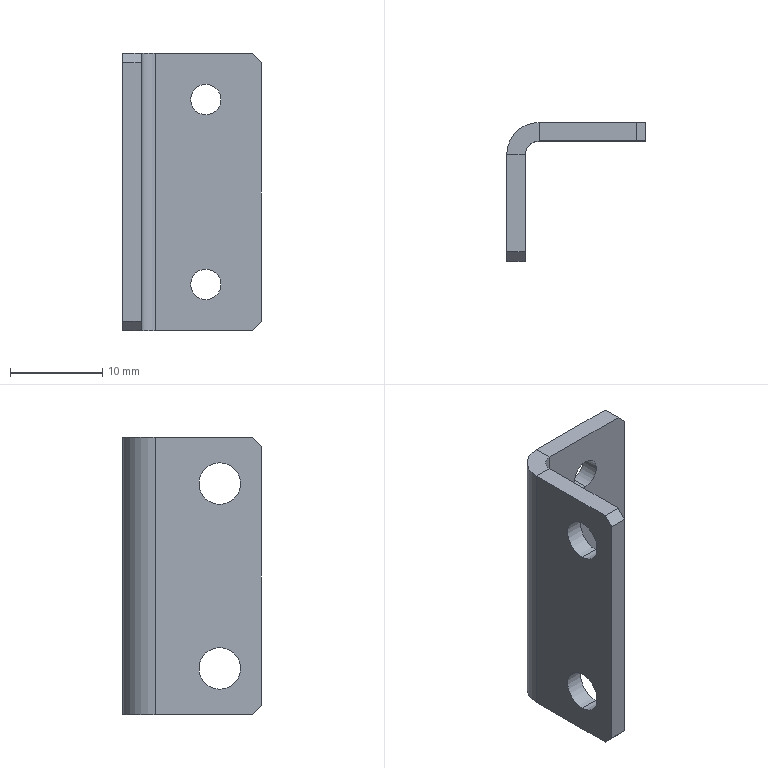Part | SolidWorks | features HoleWzd 2, Chamfer 1, FlatPattern 1, SMBaseFlange 1, SheetMetal 1 | 1 solid | 26 faces | box 15 x 15 x 30 mm | volume 1514 mm3 | plane 16 | cylinder 10 | commonest cylinder face diameters 3.3 x4 4.5 x4 3 x1 7 x1
STEP:
#1=CARTESIAN_POINT('',(2.,4.5,-12.25));
#2=VERTEX_POINT('',#1);
#3=CARTESIAN_POINT('',(2.,4.5,-7.75));
#4=VERTEX_POINT('',#3);
#5=CARTESIAN_POINT('',(2.,4.5,-10.));
#6=DIRECTION('',(-1.,0.,0.));
#7=DIRECTION('',(0.,0.,1.));
#8=AXIS2_PLACEMENT_3D('',#5,#6,#7);
#9=CIRCLE('',#8,2.25);
#10=EDGE_CURVE('',#2,#4,#9,.T.);
#11=ORIENTED_EDGE('',*,*,#10,.F.);
#12=CARTESIAN_POINT('',(0.,4.5,-12.25));
#13=VERTEX_POINT('',#12);
#14=CARTESIAN_POINT('',(0.,4.5,-12.25));
#15=DIRECTION('',(-1.,0.,0.));
#16=VECTOR('',#15,1000.);
#17=LINE('',#14,#16);
#18=EDGE_CURVE('',#2,#13,#17,.T.);
#19=ORIENTED_EDGE('',*,*,#18,.T.);
#20=CARTESIAN_POINT('',(0.,4.5,-7.75));
#21=VERTEX_POINT('',#20);
#22=CARTESIAN_POINT('',(0.,4.5,-10.));
#23=DIRECTION('',(-1.,0.,0.));
#24=DIRECTION('',(0.,0.,1.));
#25=AXIS2_PLACEMENT_3D('',#22,#23,#24);
#26=CIRCLE('',#25,2.25);
#27=EDGE_CURVE('',#13,#21,#26,.T.);
#28=ORIENTED_EDGE('',*,*,#27,.T.);
#29=CARTESIAN_POINT('',(0.,4.5,-7.75));
#30=DIRECTION('',(-1.,0.,0.));
#31=VECTOR('',#30,1000.);
#32=LINE('',#29,#31);
#33=EDGE_CURVE('',#4,#21,#32,.T.);
#34=ORIENTED_EDGE('',*,*,#33,.F.);
#35=EDGE_LOOP('',(#11,#19,#28,#34));
#36=FACE_OUTER_BOUND('',#35,.T.);
#37=CARTESIAN_POINT('',(0.,4.5,-10.));
#38=DIRECTION('',(-1.,0.,0.));
#39=DIRECTION('',(0.,0.,1.));
#40=AXIS2_PLACEMENT_3D('',#37,#38,#39);
#41=CYLINDRICAL_SURFACE('',#40,2.25);
#42=ADVANCED_FACE('',(#36),#41,.F.);
#43=CARTESIAN_POINT('',(2.,4.5,7.75));
#44=VERTEX_POINT('',#43);
#45=CARTESIAN_POINT('',(2.,4.5,12.25));
#46=VERTEX_POINT('',#45);
#47=CARTESIAN_POINT('',(2.,4.5,10.));
#48=DIRECTION('',(-1.,0.,0.));
#49=DIRECTION('',(0.,0.,1.));
#50=AXIS2_PLACEMENT_3D('',#47,#48,#49);
#51=CIRCLE('',#50,2.25);
#52=EDGE_CURVE('',#44,#46,#51,.T.);
#53=ORIENTED_EDGE('',*,*,#52,.F.);
#54=CARTESIAN_POINT('',(0.,4.5,7.75));
#55=VERTEX_POINT('',#54);
#56=CARTESIAN_POINT('',(0.,4.5,7.75));
#57=DIRECTION('',(-1.,0.,0.));
#58=VECTOR('',#57,1000.);
#59=LINE('',#56,#58);
#60=EDGE_CURVE('',#44,#55,#59,.T.);
#61=ORIENTED_EDGE('',*,*,#60,.T.);
#62=CARTESIAN_POINT('',(0.,4.5,12.25));
#63=VERTEX_POINT('',#62);
#64=CARTESIAN_POINT('',(0.,4.5,10.));
#65=DIRECTION('',(-1.,0.,0.));
#66=DIRECTION('',(0.,0.,1.));
#67=AXIS2_PLACEMENT_3D('',#64,#65,#66);
#68=CIRCLE('',#67,2.25);
#69=EDGE_CURVE('',#55,#63,#68,.T.);
#70=ORIENTED_EDGE('',*,*,#69,.T.);
#71=CARTESIAN_POINT('',(0.,4.5,12.25));
#72=DIRECTION('',(-1.,0.,0.));
#73=VECTOR('',#72,1000.);
#74=LINE('',#71,#73);
#75=EDGE_CURVE('',#46,#63,#74,.T.);
#76=ORIENTED_EDGE('',*,*,#75,.F.);
#77=EDGE_LOOP('',(#53,#61,#70,#76));
#78=FACE_OUTER_BOUND('',#77,.T.);
#79=CARTESIAN_POINT('',(0.,4.5,10.));
#80=DIRECTION('',(-1.,0.,0.));
#81=DIRECTION('',(0.,0.,1.));
#82=AXIS2_PLACEMENT_3D('',#79,#80,#81);
#83=CYLINDRICAL_SURFACE('',#82,2.25);
#84=ADVANCED_FACE('',(#78),#83,.F.);
#85=CARTESIAN_POINT('',(9.,13.,-11.65));
#86=VERTEX_POINT('',#85);
#87=CARTESIAN_POINT('',(9.,13.,-8.35));
#88=VERTEX_POINT('',#87);
#89=CARTESIAN_POINT('',(9.,13.,-10.));
#90=DIRECTION('',(0.,1.,0.));
#91=DIRECTION('',(0.,0.,1.));
#92=AXIS2_PLACEMENT_3D('',#89,#90,#91);
#93=CIRCLE('',#92,1.65);
#94=EDGE_CURVE('',#86,#88,#93,.T.);
#95=ORIENTED_EDGE('',*,*,#94,.F.);
#96=CARTESIAN_POINT('',(9.,15.,-11.65));
#97=VERTEX_POINT('',#96);
#98=CARTESIAN_POINT('',(9.,15.,-11.65));
#99=DIRECTION('',(0.,1.,0.));
#100=VECTOR('',#99,1000.);
#101=LINE('',#98,#100);
#102=EDGE_CURVE('',#86,#97,#101,.T.);
#103=ORIENTED_EDGE('',*,*,#102,.T.);
#104=CARTESIAN_POINT('',(9.,15.,-8.35));
#105=VERTEX_POINT('',#104);
#106=CARTESIAN_POINT('',(9.,15.,-10.));
#107=DIRECTION('',(0.,1.,0.));
#108=DIRECTION('',(0.,0.,1.));
#109=AXIS2_PLACEMENT_3D('',#106,#107,#108);
#110=CIRCLE('',#109,1.65);
#111=EDGE_CURVE('',#97,#105,#110,.T.);
#112=ORIENTED_EDGE('',*,*,#111,.T.);
#113=CARTESIAN_POINT('',(9.,15.,-8.35));
#114=DIRECTION('',(0.,1.,0.));
#115=VECTOR('',#114,1000.);
#116=LINE('',#113,#115);
#117=EDGE_CURVE('',#88,#105,#116,.T.);
#118=ORIENTED_EDGE('',*,*,#117,.F.);
#119=EDGE_LOOP('',(#95,#103,#112,#118));
#120=FACE_OUTER_BOUND('',#119,.T.);
#121=CARTESIAN_POINT('',(9.,15.,-10.));
#122=DIRECTION('',(0.,1.,0.));
#123=DIRECTION('',(0.,0.,1.));
#124=AXIS2_PLACEMENT_3D('',#121,#122,#123);
#125=CYLINDRICAL_SURFACE('',#124,1.65);
#126=ADVANCED_FACE('',(#120),#125,.F.);
#127=CARTESIAN_POINT('',(9.,13.,8.35));
#128=VERTEX_POINT('',#127);
#129=CARTESIAN_POINT('',(9.,13.,11.65));
#130=VERTEX_POINT('',#129);
#131=CARTESIAN_POINT('',(9.,13.,10.));
#132=DIRECTION('',(0.,1.,0.));
#133=DIRECTION('',(0.,0.,1.));
#134=AXIS2_PLACEMENT_3D('',#131,#132,#133);
#135=CIRCLE('',#134,1.65);
#136=EDGE_CURVE('',#128,#130,#135,.T.);
#137=ORIENTED_EDGE('',*,*,#136,.F.);
#138=CARTESIAN_POINT('',(9.,15.,8.35));
#139=VERTEX_POINT('',#138);
#140=CARTESIAN_POINT('',(9.,15.,8.35));
#141=DIRECTION('',(0.,1.,0.));
#142=VECTOR('',#141,1000.);
#143=LINE('',#140,#142);
#144=EDGE_CURVE('',#128,#139,#143,.T.);
#145=ORIENTED_EDGE('',*,*,#144,.T.);
#146=CARTESIAN_POINT('',(9.,15.,11.65));
#147=VERTEX_POINT('',#146);
#148=CARTESIAN_POINT('',(9.,15.,10.));
#149=DIRECTION('',(0.,1.,0.));
#150=DIRECTION('',(0.,0.,1.));
#151=AXIS2_PLACEMENT_3D('',#148,#149,#150);
#152=CIRCLE('',#151,1.65);
#153=EDGE_CURVE('',#139,#147,#152,.T.);
#154=ORIENTED_EDGE('',*,*,#153,.T.);
#155=CARTESIAN_POINT('',(9.,15.,11.65));
#156=DIRECTION('',(0.,1.,0.));
#157=VECTOR('',#156,1000.);
#158=LINE('',#155,#157);
#159=EDGE_CURVE('',#130,#147,#158,.T.);
#160=ORIENTED_EDGE('',*,*,#159,.F.);
#161=EDGE_LOOP('',(#137,#145,#154,#160));
#162=FACE_OUTER_BOUND('',#161,.T.);
#163=CARTESIAN_POINT('',(9.,15.,10.));
#164=DIRECTION('',(0.,1.,0.));
#165=DIRECTION('',(0.,0.,1.));
#166=AXIS2_PLACEMENT_3D('',#163,#164,#165);
#167=CYLINDRICAL_SURFACE('',#166,1.65);
#168=ADVANCED_FACE('',(#162),#167,.F.);
#169=CARTESIAN_POINT('',(3.5,15.,15.));
#170=VERTEX_POINT('',#169);
#171=CARTESIAN_POINT('',(3.5,13.,15.));
#172=VERTEX_POINT('',#171);
#173=CARTESIAN_POINT('',(3.5,15.,15.));
#174=DIRECTION('',(0.,-1.,0.));
#175=VECTOR('',#174,1000.);
#176=LINE('',#173,#175);
#177=EDGE_CURVE('',#170,#172,#176,.T.);
#178=ORIENTED_EDGE('',*,*,#177,.F.);
#179=CARTESIAN_POINT('',(0.,11.5,15.));
#180=VERTEX_POINT('',#179);
#181=CARTESIAN_POINT('',(3.5,11.5,15.));
#182=DIRECTION('',(0.,0.,-1.));
#183=DIRECTION('',(1.,0.,0.));
#184=AXIS2_PLACEMENT_3D('',#181,#182,#183);
#185=CIRCLE('',#184,3.5);
#186=EDGE_CURVE('',#180,#170,#185,.T.);
#187=ORIENTED_EDGE('',*,*,#186,.F.);
#188=CARTESIAN_POINT('',(2.,11.5,15.));
#189=VERTEX_POINT('',#188);
#190=CARTESIAN_POINT('',(2.,11.5,15.));
#191=DIRECTION('',(-1.,0.,0.));
#192=VECTOR('',#191,1000.);
#193=LINE('',#190,#192);
#194=EDGE_CURVE('',#189,#180,#193,.T.);
#195=ORIENTED_EDGE('',*,*,#194,.F.);
#196=CARTESIAN_POINT('',(3.5,11.5,15.));
#197=DIRECTION('',(0.,0.,-1.));
#198=DIRECTION('',(1.,0.,0.));
#199=AXIS2_PLACEMENT_3D('',#196,#197,#198);
#200=CIRCLE('',#199,1.5);
#201=EDGE_CURVE('',#189,#172,#200,.T.);
#202=ORIENTED_EDGE('',*,*,#201,.T.);
#203=EDGE_LOOP('',(#178,#187,#195,#202));
#204=FACE_OUTER_BOUND('',#203,.T.);
#205=CARTESIAN_POINT('',(3.5,15.,15.));
#206=DIRECTION('',(0.,0.,1.));
#207=DIRECTION('',(1.,0.,0.));
#208=AXIS2_PLACEMENT_3D('',#205,#206,#207);
#209=PLANE('',#208);
#210=ADVANCED_FACE('',(#204),#209,.T.);
#211=CARTESIAN_POINT('',(14.,13.,15.));
#212=VERTEX_POINT('',#211);
#213=CARTESIAN_POINT('',(0.,13.,15.));
#214=DIRECTION('',(1.,0.,0.));
#215=VECTOR('',#214,1000.);
#216=LINE('',#213,#215);
#217=EDGE_CURVE('',#172,#212,#216,.T.);
#218=ORIENTED_EDGE('',*,*,#217,.T.);
#219=CARTESIAN_POINT('',(14.,15.,15.));
#220=VERTEX_POINT('',#219);
#221=CARTESIAN_POINT('',(14.,11.5,15.));
#222=DIRECTION('',(0.,1.,0.));
#223=VECTOR('',#222,1000.);
#224=LINE('',#221,#223);
#225=EDGE_CURVE('',#212,#220,#224,.T.);
#226=ORIENTED_EDGE('',*,*,#225,.T.);
#227=CARTESIAN_POINT('',(0.,15.,15.));
#228=DIRECTION('',(1.,0.,0.));
#229=VECTOR('',#228,1000.);
#230=LINE('',#227,#229);
#231=EDGE_CURVE('',#170,#220,#230,.T.);
#232=ORIENTED_EDGE('',*,*,#231,.F.);
#233=ORIENTED_EDGE('',*,*,#177,.T.);
#234=EDGE_LOOP('',(#218,#226,#232,#233));
#235=FACE_OUTER_BOUND('',#234,.T.);
#236=CARTESIAN_POINT('',(2.,11.5,15.));
#237=DIRECTION('',(0.,0.,1.));
#238=DIRECTION('',(1.,0.,0.));
#239=AXIS2_PLACEMENT_3D('',#236,#237,#238);
#240=PLANE('',#239);
#241=ADVANCED_FACE('',(#235),#240,.T.);
#242=CARTESIAN_POINT('',(0.,11.5,-15.));
#243=VERTEX_POINT('',#242);
#244=CARTESIAN_POINT('',(2.,11.5,-15.));
#245=VERTEX_POINT('',#244);
#246=CARTESIAN_POINT('',(0.,11.5,-15.));
#247=DIRECTION('',(1.,0.,0.));
#248=VECTOR('',#247,1000.);
#249=LINE('',#246,#248);
#250=EDGE_CURVE('',#243,#245,#249,.T.);
#251=ORIENTED_EDGE('',*,*,#250,.F.);
#252=CARTESIAN_POINT('',(3.5,15.,-15.));
#253=VERTEX_POINT('',#252);
#254=CARTESIAN_POINT('',(3.5,11.5,-15.));
#255=DIRECTION('',(0.,0.,-1.));
#256=DIRECTION('',(1.,0.,0.));
#257=AXIS2_PLACEMENT_3D('',#254,#255,#256);
#258=CIRCLE('',#257,3.5);
#259=EDGE_CURVE('',#243,#253,#258,.T.);
#260=ORIENTED_EDGE('',*,*,#259,.T.);
#261=CARTESIAN_POINT('',(3.5,13.,-15.));
#262=VERTEX_POINT('',#261);
#263=CARTESIAN_POINT('',(3.5,13.,-15.));
#264=DIRECTION('',(0.,1.,0.));
#265=VECTOR('',#264,1000.);
#266=LINE('',#263,#265);
#267=EDGE_CURVE('',#262,#253,#266,.T.);
#268=ORIENTED_EDGE('',*,*,#267,.F.);
#269=CARTESIAN_POINT('',(3.5,11.5,-15.));
#270=DIRECTION('',(0.,0.,-1.));
#271=DIRECTION('',(1.,0.,0.));
#272=AXIS2_PLACEMENT_3D('',#269,#270,#271);
#273=CIRCLE('',#272,1.5);
#274=EDGE_CURVE('',#245,#262,#273,.T.);
#275=ORIENTED_EDGE('',*,*,#274,.F.);
#276=EDGE_LOOP('',(#251,#260,#268,#275));
#277=FACE_OUTER_BOUND('',#276,.T.);
#278=CARTESIAN_POINT('',(0.,11.5,-15.));
#279=DIRECTION('',(0.,0.,-1.));
#280=DIRECTION('',(-1.,0.,0.));
#281=AXIS2_PLACEMENT_3D('',#278,#279,#280);
#282=PLANE('',#281);
#283=ADVANCED_FACE('',(#277),#282,.T.);
#284=CARTESIAN_POINT('',(2.,1.,-15.));
#285=VERTEX_POINT('',#284);
#286=CARTESIAN_POINT('',(2.,0.,-15.));
#287=DIRECTION('',(0.,1.,0.));
#288=VECTOR('',#287,1000.);
#289=LINE('',#286,#288);
#290=EDGE_CURVE('',#285,#245,#289,.T.);
#291=ORIENTED_EDGE('',*,*,#290,.F.);
#292=CARTESIAN_POINT('',(0.,1.,-15.));
#293=VERTEX_POINT('',#292);
#294=CARTESIAN_POINT('',(3.5,1.,-15.));
#295=DIRECTION('',(-1.,0.,0.));
#296=VECTOR('',#295,1000.);
#297=LINE('',#294,#296);
#298=EDGE_CURVE('',#285,#293,#297,.T.);
#299=ORIENTED_EDGE('',*,*,#298,.T.);
#300=CARTESIAN_POINT('',(0.,0.,-15.));
#301=DIRECTION('',(0.,1.,0.));
#302=VECTOR('',#301,1000.);
#303=LINE('',#300,#302);
#304=EDGE_CURVE('',#293,#243,#303,.T.);
#305=ORIENTED_EDGE('',*,*,#304,.T.);
#306=ORIENTED_EDGE('',*,*,#250,.T.);
#307=EDGE_LOOP('',(#291,#299,#305,#306));
#308=FACE_OUTER_BOUND('',#307,.T.);
#309=CARTESIAN_POINT('',(3.5,13.,-15.));
#310=DIRECTION('',(0.,0.,-1.));
#311=DIRECTION('',(-1.,0.,0.));
#312=AXIS2_PLACEMENT_3D('',#309,#310,#311);
#313=PLANE('',#312);
#314=ADVANCED_FACE('',(#308),#313,.T.);
#315=CARTESIAN_POINT('',(9.,13.,-10.));
#316=DIRECTION('',(0.,1.,0.));
#317=DIRECTION('',(0.,0.,1.));
#318=AXIS2_PLACEMENT_3D('',#315,#316,#317);
#319=CIRCLE('',#318,1.65);
#320=EDGE_CURVE('',#88,#86,#319,.T.);
#321=ORIENTED_EDGE('',*,*,#320,.T.);
#322=ORIENTED_EDGE('',*,*,#94,.T.);
#323=EDGE_LOOP('',(#321,#322));
#324=FACE_BOUND('',#323,.T.);
#325=CARTESIAN_POINT('',(9.,13.,10.));
#326=DIRECTION('',(0.,1.,0.));
#327=DIRECTION('',(0.,0.,1.));
#328=AXIS2_PLACEMENT_3D('',#325,#326,#327);
#329=CIRCLE('',#328,1.65);
#330=EDGE_CURVE('',#130,#128,#329,.T.);
#331=ORIENTED_EDGE('',*,*,#330,.T.);
#332=ORIENTED_EDGE('',*,*,#136,.T.);
#333=EDGE_LOOP('',(#331,#332));
#334=FACE_BOUND('',#333,.T.);
#335=CARTESIAN_POINT('',(14.,13.,-15.));
#336=VERTEX_POINT('',#335);
#337=CARTESIAN_POINT('',(0.,13.,-15.));
#338=DIRECTION('',(1.,0.,0.));
#339=VECTOR('',#338,1000.);
#340=LINE('',#337,#339);
#341=EDGE_CURVE('',#262,#336,#340,.T.);
#342=ORIENTED_EDGE('',*,*,#341,.T.);
#343=CARTESIAN_POINT('',(15.,13.,-14.));
#344=VERTEX_POINT('',#343);
#345=CARTESIAN_POINT('',(14.,13.,-15.));
#346=DIRECTION('',(0.7071,0.,0.7071));
#347=VECTOR('',#346,1000.);
#348=LINE('',#345,#347);
#349=EDGE_CURVE('',#336,#344,#348,.T.);
#350=ORIENTED_EDGE('',*,*,#349,.T.);
#351=CARTESIAN_POINT('',(15.,13.,14.));
#352=VERTEX_POINT('',#351);
#353=CARTESIAN_POINT('',(15.,13.,15.));
#354=DIRECTION('',(0.,0.,-1.));
#355=VECTOR('',#354,1000.);
#356=LINE('',#353,#355);
#357=EDGE_CURVE('',#352,#344,#356,.T.);
#358=ORIENTED_EDGE('',*,*,#357,.F.);
#359=CARTESIAN_POINT('',(15.,13.,14.));
#360=DIRECTION('',(-0.7071,0.,0.7071));
#361=VECTOR('',#360,1000.);
#362=LINE('',#359,#361);
#363=EDGE_CURVE('',#352,#212,#362,.T.);
#364=ORIENTED_EDGE('',*,*,#363,.T.);
#365=ORIENTED_EDGE('',*,*,#217,.F.);
#366=CARTESIAN_POINT('',(3.5,13.,15.));
#367=DIRECTION('',(0.,0.,-1.));
#368=VECTOR('',#367,1000.);
#369=LINE('',#366,#368);
#370=EDGE_CURVE('',#172,#262,#369,.T.);
#371=ORIENTED_EDGE('',*,*,#370,.T.);
#372=EDGE_LOOP('',(#342,#350,#358,#364,#365,#371));
#373=FACE_OUTER_BOUND('',#372,.T.);
#374=CARTESIAN_POINT('',(0.,13.,15.));
#375=DIRECTION('',(0.,1.,0.));
#376=DIRECTION('',(0.,0.,1.));
#377=AXIS2_PLACEMENT_3D('',#374,#375,#376);
#378=PLANE('',#377);
#379=ADVANCED_FACE('',(#324,#334,#373),#378,.F.);
#380=ORIENTED_EDGE('',*,*,#357,.T.);
#381=CARTESIAN_POINT('',(15.,15.,-14.));
#382=VERTEX_POINT('',#381);
#383=CARTESIAN_POINT('',(15.,15.,-14.));
#384=DIRECTION('',(0.,1.,0.));
#385=VECTOR('',#384,1000.);
#386=LINE('',#383,#385);
#387=EDGE_CURVE('',#344,#382,#386,.T.);
#388=ORIENTED_EDGE('',*,*,#387,.T.);
#389=CARTESIAN_POINT('',(15.,15.,14.));
#390=VERTEX_POINT('',#389);
#391=CARTESIAN_POINT('',(15.,15.,15.));
#392=DIRECTION('',(0.,0.,-1.));
#393=VECTOR('',#392,1000.);
#394=LINE('',#391,#393);
#395=EDGE_CURVE('',#390,#382,#394,.T.);
#396=ORIENTED_EDGE('',*,*,#395,.F.);
#397=CARTESIAN_POINT('',(15.,15.,14.));
#398=DIRECTION('',(0.,-1.,0.));
#399=VECTOR('',#398,1000.);
#400=LINE('',#397,#399);
#401=EDGE_CURVE('',#390,#352,#400,.T.);
#402=ORIENTED_EDGE('',*,*,#401,.T.);
#403=EDGE_LOOP('',(#380,#388,#396,#402));
#404=FACE_OUTER_BOUND('',#403,.T.);
#405=CARTESIAN_POINT('',(15.,15.,15.));
#406=DIRECTION('',(1.,0.,0.));
#407=DIRECTION('',(0.,0.,-1.));
#408=AXIS2_PLACEMENT_3D('',#405,#406,#407);
#409=PLANE('',#408);
#410=ADVANCED_FACE('',(#404),#409,.T.);
#411=CARTESIAN_POINT('',(9.,15.,-10.));
#412=DIRECTION('',(0.,1.,0.));
#413=DIRECTION('',(0.,0.,1.));
#414=AXIS2_PLACEMENT_3D('',#411,#412,#413);
#415=CIRCLE('',#414,1.65);
#416=EDGE_CURVE('',#105,#97,#415,.T.);
#417=ORIENTED_EDGE('',*,*,#416,.F.);
#418=ORIENTED_EDGE('',*,*,#111,.F.);
#419=EDGE_LOOP('',(#417,#418));
#420=FACE_BOUND('',#419,.T.);
#421=CARTESIAN_POINT('',(9.,15.,10.));
#422=DIRECTION('',(0.,1.,0.));
#423=DIRECTION('',(0.,0.,1.));
#424=AXIS2_PLACEMENT_3D('',#421,#422,#423);
#425=CIRCLE('',#424,1.65);
#426=EDGE_CURVE('',#147,#139,#425,.T.);
#427=ORIENTED_EDGE('',*,*,#426,.F.);
#428=ORIENTED_EDGE('',*,*,#153,.F.);
#429=EDGE_LOOP('',(#427,#428));
#430=FACE_BOUND('',#429,.T.);
#431=ORIENTED_EDGE('',*,*,#395,.T.);
#432=CARTESIAN_POINT('',(14.,15.,-15.));
#433=VERTEX_POINT('',#432);
#434=CARTESIAN_POINT('',(22.,15.,-7.));
#435=DIRECTION('',(-0.7071,0.,-0.7071));
#436=VECTOR('',#435,1000.);
#437=LINE('',#434,#436);
#438=EDGE_CURVE('',#382,#433,#437,.T.);
#439=ORIENTED_EDGE('',*,*,#438,.T.);
#440=CARTESIAN_POINT('',(0.,15.,-15.));
#441=DIRECTION('',(1.,0.,0.));
#442=VECTOR('',#441,1000.);
#443=LINE('',#440,#442);
#444=EDGE_CURVE('',#253,#433,#443,.T.);
#445=ORIENTED_EDGE('',*,*,#444,.F.);
#446=CARTESIAN_POINT('',(3.5,15.,15.));
#447=DIRECTION('',(0.,0.,-1.));
#448=VECTOR('',#447,1000.);
#449=LINE('',#446,#448);
#450=EDGE_CURVE('',#170,#253,#449,.T.);
#451=ORIENTED_EDGE('',*,*,#450,.F.);
#452=ORIENTED_EDGE('',*,*,#231,.T.);
#453=CARTESIAN_POINT('',(7.,15.,22.));
#454=DIRECTION('',(0.7071,0.,-0.7071));
#455=VECTOR('',#454,1000.);
#456=LINE('',#453,#455);
#457=EDGE_CURVE('',#220,#390,#456,.T.);
#458=ORIENTED_EDGE('',*,*,#457,.T.);
#459=EDGE_LOOP('',(#431,#439,#445,#451,#452,#458));
#460=FACE_OUTER_BOUND('',#459,.T.);
#461=CARTESIAN_POINT('',(0.,15.,15.));
#462=DIRECTION('',(0.,1.,0.));
#463=DIRECTION('',(0.,0.,1.));
#464=AXIS2_PLACEMENT_3D('',#461,#462,#463);
#465=PLANE('',#464);
#466=ADVANCED_FACE('',(#420,#430,#460),#465,.T.);
#467=ORIENTED_EDGE('',*,*,#259,.F.);
#468=CARTESIAN_POINT('',(0.,11.5,15.));
#469=DIRECTION('',(0.,0.,-1.));
#470=VECTOR('',#469,1000.);
#471=LINE('',#468,#470);
#472=EDGE_CURVE('',#180,#243,#471,.T.);
#473=ORIENTED_EDGE('',*,*,#472,.F.);
#474=ORIENTED_EDGE('',*,*,#186,.T.);
#475=ORIENTED_EDGE('',*,*,#450,.T.);
#476=EDGE_LOOP('',(#467,#473,#474,#475));
#477=FACE_OUTER_BOUND('',#476,.T.);
#478=CARTESIAN_POINT('',(3.5,11.5,15.));
#479=DIRECTION('',(0.,0.,-1.));
#480=DIRECTION('',(-1.,0.,0.));
#481=AXIS2_PLACEMENT_3D('',#478,#479,#480);
#482=CYLINDRICAL_SURFACE('',#481,3.5);
#483=ADVANCED_FACE('',(#477),#482,.T.);
#484=CARTESIAN_POINT('',(0.,4.5,-10.));
#485=DIRECTION('',(-1.,0.,0.));
#486=DIRECTION('',(0.,0.,1.));
#487=AXIS2_PLACEMENT_3D('',#484,#485,#486);
#488=CIRCLE('',#487,2.25);
#489=EDGE_CURVE('',#21,#13,#488,.T.);
#490=ORIENTED_EDGE('',*,*,#489,.F.);
#491=ORIENTED_EDGE('',*,*,#27,.F.);
#492=EDGE_LOOP('',(#490,#491));
#493=FACE_BOUND('',#492,.T.);
#494=CARTESIAN_POINT('',(0.,4.5,10.));
#495=DIRECTION('',(-1.,0.,0.));
#496=DIRECTION('',(0.,0.,1.));
#497=AXIS2_PLACEMENT_3D('',#494,#495,#496);
#498=CIRCLE('',#497,2.25);
#499=EDGE_CURVE('',#63,#55,#498,.T.);
#500=ORIENTED_EDGE('',*,*,#499,.F.);
#501=ORIENTED_EDGE('',*,*,#69,.F.);
#502=EDGE_LOOP('',(#500,#501));
#503=FACE_BOUND('',#502,.T.);
#504=ORIENTED_EDGE('',*,*,#304,.F.);
#505=CARTESIAN_POINT('',(0.,0.,-14.));
#506=VERTEX_POINT('',#505);
#507=CARTESIAN_POINT('',(0.,-14.5,0.5));
#508=DIRECTION('',(0.,-0.7071,0.7071));
#509=VECTOR('',#508,1000.);
#510=LINE('',#507,#509);
#511=EDGE_CURVE('',#293,#506,#510,.T.);
#512=ORIENTED_EDGE('',*,*,#511,.T.);
#513=CARTESIAN_POINT('',(0.,0.,14.));
#514=VERTEX_POINT('',#513);
#515=CARTESIAN_POINT('',(0.,0.,15.));
#516=DIRECTION('',(0.,0.,-1.));
#517=VECTOR('',#516,1000.);
#518=LINE('',#515,#517);
#519=EDGE_CURVE('',#514,#506,#518,.T.);
#520=ORIENTED_EDGE('',*,*,#519,.F.);
#521=CARTESIAN_POINT('',(0.,1.,15.));
#522=VERTEX_POINT('',#521);
#523=CARTESIAN_POINT('',(0.,0.5,14.5));
#524=DIRECTION('',(0.,0.7071,0.7071));
#525=VECTOR('',#524,1000.);
#526=LINE('',#523,#525);
#527=EDGE_CURVE('',#514,#522,#526,.T.);
#528=ORIENTED_EDGE('',*,*,#527,.T.);
#529=CARTESIAN_POINT('',(0.,0.,15.));
#530=DIRECTION('',(0.,1.,0.));
#531=VECTOR('',#530,1000.);
#532=LINE('',#529,#531);
#533=EDGE_CURVE('',#522,#180,#532,.T.);
#534=ORIENTED_EDGE('',*,*,#533,.T.);
#535=ORIENTED_EDGE('',*,*,#472,.T.);
#536=EDGE_LOOP('',(#504,#512,#520,#528,#534,#535));
#537=FACE_OUTER_BOUND('',#536,.T.);
#538=CARTESIAN_POINT('',(0.,0.,15.));
#539=DIRECTION('',(-1.,0.,0.));
#540=DIRECTION('',(0.,0.,1.));
#541=AXIS2_PLACEMENT_3D('',#538,#539,#540);
#542=PLANE('',#541);
#543=ADVANCED_FACE('',(#493,#503,#537),#542,.T.);
#544=ORIENTED_EDGE('',*,*,#519,.T.);
#545=CARTESIAN_POINT('',(2.,0.,-14.));
#546=VERTEX_POINT('',#545);
#547=CARTESIAN_POINT('',(2.,0.,-14.));
#548=DIRECTION('',(1.,0.,0.));
#549=VECTOR('',#548,1000.);
#550=LINE('',#547,#549);
#551=EDGE_CURVE('',#506,#546,#550,.T.);
#552=ORIENTED_EDGE('',*,*,#551,.T.);
#553=CARTESIAN_POINT('',(2.,0.,14.));
#554=VERTEX_POINT('',#553);
#555=CARTESIAN_POINT('',(2.,0.,15.));
#556=DIRECTION('',(0.,0.,-1.));
#557=VECTOR('',#556,1000.);
#558=LINE('',#555,#557);
#559=EDGE_CURVE('',#554,#546,#558,.T.);
#560=ORIENTED_EDGE('',*,*,#559,.F.);
#561=CARTESIAN_POINT('',(2.,0.,14.));
#562=DIRECTION('',(-1.,0.,0.));
#563=VECTOR('',#562,1000.);
#564=LINE('',#561,#563);
#565=EDGE_CURVE('',#554,#514,#564,.T.);
#566=ORIENTED_EDGE('',*,*,#565,.T.);
#567=EDGE_LOOP('',(#544,#552,#560,#566));
#568=FACE_OUTER_BOUND('',#567,.T.);
#569=CARTESIAN_POINT('',(2.,0.,15.));
#570=DIRECTION('',(0.,-1.,0.));
#571=DIRECTION('',(0.,0.,-1.));
#572=AXIS2_PLACEMENT_3D('',#569,#570,#571);
#573=PLANE('',#572);
#574=ADVANCED_FACE('',(#568),#573,.T.);
#575=CARTESIAN_POINT('',(2.,4.5,-10.));
#576=DIRECTION('',(-1.,0.,0.));
#577=DIRECTION('',(0.,0.,1.));
#578=AXIS2_PLACEMENT_3D('',#575,#576,#577);
#579=CIRCLE('',#578,2.25);
#580=EDGE_CURVE('',#4,#2,#579,.T.);
#581=ORIENTED_EDGE('',*,*,#580,.T.);
#582=ORIENTED_EDGE('',*,*,#10,.T.);
#583=EDGE_LOOP('',(#581,#582));
#584=FACE_BOUND('',#583,.T.);
#585=CARTESIAN_POINT('',(2.,4.5,10.));
#586=DIRECTION('',(-1.,0.,0.));
#587=DIRECTION('',(0.,0.,1.));
#588=AXIS2_PLACEMENT_3D('',#585,#586,#587);
#589=CIRCLE('',#588,2.25);
#590=EDGE_CURVE('',#46,#44,#589,.T.);
#591=ORIENTED_EDGE('',*,*,#590,.T.);
#592=ORIENTED_EDGE('',*,*,#52,.T.);
#593=EDGE_LOOP('',(#591,#592));
#594=FACE_BOUND('',#593,.T.);
#595=ORIENTED_EDGE('',*,*,#559,.T.);
#596=CARTESIAN_POINT('',(2.,1.,-15.));
#597=DIRECTION('',(0.,0.7071,-0.7071));
#598=VECTOR('',#597,1000.);
#599=LINE('',#596,#598);
#600=EDGE_CURVE('',#546,#285,#599,.T.);
#601=ORIENTED_EDGE('',*,*,#600,.T.);
#602=ORIENTED_EDGE('',*,*,#290,.T.);
#603=CARTESIAN_POINT('',(2.,11.5,15.));
#604=DIRECTION('',(0.,0.,-1.));
#605=VECTOR('',#604,1000.);
#606=LINE('',#603,#605);
#607=EDGE_CURVE('',#189,#245,#606,.T.);
#608=ORIENTED_EDGE('',*,*,#607,.F.);
#609=CARTESIAN_POINT('',(2.,1.,15.));
#610=VERTEX_POINT('',#609);
#611=CARTESIAN_POINT('',(2.,0.,15.));
#612=DIRECTION('',(0.,1.,0.));
#613=VECTOR('',#612,1000.);
#614=LINE('',#611,#613);
#615=EDGE_CURVE('',#610,#189,#614,.T.);
#616=ORIENTED_EDGE('',*,*,#615,.F.);
#617=CARTESIAN_POINT('',(2.,0.,14.));
#618=DIRECTION('',(0.,-0.7071,-0.7071));
#619=VECTOR('',#618,1000.);
#620=LINE('',#617,#619);
#621=EDGE_CURVE('',#610,#554,#620,.T.);
#622=ORIENTED_EDGE('',*,*,#621,.T.);
#623=EDGE_LOOP('',(#595,#601,#602,#608,#616,#622));
#624=FACE_OUTER_BOUND('',#623,.T.);
#625=CARTESIAN_POINT('',(2.,0.,15.));
#626=DIRECTION('',(-1.,0.,0.));
#627=DIRECTION('',(0.,0.,1.));
#628=AXIS2_PLACEMENT_3D('',#625,#626,#627);
#629=PLANE('',#628);
#630=ADVANCED_FACE('',(#584,#594,#624),#629,.F.);
#631=ORIENTED_EDGE('',*,*,#274,.T.);
#632=ORIENTED_EDGE('',*,*,#370,.F.);
#633=ORIENTED_EDGE('',*,*,#201,.F.);
#634=ORIENTED_EDGE('',*,*,#607,.T.);
#635=EDGE_LOOP('',(#631,#632,#633,#634));
#636=FACE_OUTER_BOUND('',#635,.T.);
#637=CARTESIAN_POINT('',(3.5,11.5,15.));
#638=DIRECTION('',(0.,0.,-1.));
#639=DIRECTION('',(-1.,0.,0.));
#640=AXIS2_PLACEMENT_3D('',#637,#638,#639);
#641=CYLINDRICAL_SURFACE('',#640,1.5);
#642=ADVANCED_FACE('',(#636),#641,.F.);
#643=ORIENTED_EDGE('',*,*,#533,.F.);
#644=CARTESIAN_POINT('',(3.5,1.,15.));
#645=DIRECTION('',(1.,0.,0.));
#646=VECTOR('',#645,1000.);
#647=LINE('',#644,#646);
#648=EDGE_CURVE('',#522,#610,#647,.T.);
#649=ORIENTED_EDGE('',*,*,#648,.T.);
#650=ORIENTED_EDGE('',*,*,#615,.T.);
#651=ORIENTED_EDGE('',*,*,#194,.T.);
#652=EDGE_LOOP('',(#643,#649,#650,#651));
#653=FACE_OUTER_BOUND('',#652,.T.);
#654=CARTESIAN_POINT('',(3.5,11.5,15.));
#655=DIRECTION('',(0.,0.,1.));
#656=DIRECTION('',(1.,0.,0.));
#657=AXIS2_PLACEMENT_3D('',#654,#655,#656);
#658=PLANE('',#657);
#659=ADVANCED_FACE('',(#653),#658,.T.);
#660=ORIENTED_EDGE('',*,*,#444,.T.);
#661=CARTESIAN_POINT('',(14.,13.,-15.));
#662=DIRECTION('',(0.,-1.,0.));
#663=VECTOR('',#662,1000.);
#664=LINE('',#661,#663);
#665=EDGE_CURVE('',#433,#336,#664,.T.);
#666=ORIENTED_EDGE('',*,*,#665,.T.);
#667=ORIENTED_EDGE('',*,*,#341,.F.);
#668=ORIENTED_EDGE('',*,*,#267,.T.);
#669=EDGE_LOOP('',(#660,#666,#667,#668));
#670=FACE_OUTER_BOUND('',#669,.T.);
#671=CARTESIAN_POINT('',(3.5,11.5,-15.));
#672=DIRECTION('',(0.,0.,1.));
#673=DIRECTION('',(1.,0.,0.));
#674=AXIS2_PLACEMENT_3D('',#671,#672,#673);
#675=PLANE('',#674);
#676=ADVANCED_FACE('',(#670),#675,.F.);
#677=ORIENTED_EDGE('',*,*,#600,.F.);
#678=ORIENTED_EDGE('',*,*,#551,.F.);
#679=ORIENTED_EDGE('',*,*,#511,.F.);
#680=ORIENTED_EDGE('',*,*,#298,.F.);
#681=EDGE_LOOP('',(#677,#678,#679,#680));
#682=FACE_OUTER_BOUND('',#681,.T.);
#683=CARTESIAN_POINT('',(3.5,1.,-15.));
#684=DIRECTION('',(0.,0.7071,0.7071));
#685=DIRECTION('',(-1.,0.,0.));
#686=AXIS2_PLACEMENT_3D('',#683,#684,#685);
#687=PLANE('',#686);
#688=ADVANCED_FACE('',(#682),#687,.F.);
#689=ORIENTED_EDGE('',*,*,#621,.F.);
#690=ORIENTED_EDGE('',*,*,#648,.F.);
#691=ORIENTED_EDGE('',*,*,#527,.F.);
#692=ORIENTED_EDGE('',*,*,#565,.F.);
#693=EDGE_LOOP('',(#689,#690,#691,#692));
#694=FACE_OUTER_BOUND('',#693,.T.);
#695=CARTESIAN_POINT('',(2.,0.,14.));
#696=DIRECTION('',(0.,0.7071,-0.7071));
#697=DIRECTION('',(-1.,0.,0.));
#698=AXIS2_PLACEMENT_3D('',#695,#696,#697);
#699=PLANE('',#698);
#700=ADVANCED_FACE('',(#694),#699,.F.);
#701=ORIENTED_EDGE('',*,*,#438,.F.);
#702=ORIENTED_EDGE('',*,*,#387,.F.);
#703=ORIENTED_EDGE('',*,*,#349,.F.);
#704=ORIENTED_EDGE('',*,*,#665,.F.);
#705=EDGE_LOOP('',(#701,#702,#703,#704));
#706=FACE_OUTER_BOUND('',#705,.T.);
#707=CARTESIAN_POINT('',(14.,11.5,-15.));
#708=DIRECTION('',(0.7071,0.,-0.7071));
#709=DIRECTION('',(0.,1.,0.));
#710=AXIS2_PLACEMENT_3D('',#707,#708,#709);
#711=PLANE('',#710);
#712=ADVANCED_FACE('',(#706),#711,.T.);
#713=ORIENTED_EDGE('',*,*,#457,.F.);
#714=ORIENTED_EDGE('',*,*,#225,.F.);
#715=ORIENTED_EDGE('',*,*,#363,.F.);
#716=ORIENTED_EDGE('',*,*,#401,.F.);
#717=EDGE_LOOP('',(#713,#714,#715,#716));
#718=FACE_OUTER_BOUND('',#717,.T.);
#719=CARTESIAN_POINT('',(15.,15.,14.));
#720=DIRECTION('',(-0.7071,0.,-0.7071));
#721=DIRECTION('',(0.,-1.,0.));
#722=AXIS2_PLACEMENT_3D('',#719,#720,#721);
#723=PLANE('',#722);
#724=ADVANCED_FACE('',(#718),#723,.F.);
#725=ORIENTED_EDGE('',*,*,#144,.F.);
#726=ORIENTED_EDGE('',*,*,#330,.F.);
#727=ORIENTED_EDGE('',*,*,#159,.T.);
#728=ORIENTED_EDGE('',*,*,#426,.T.);
#729=EDGE_LOOP('',(#725,#726,#727,#728));
#730=FACE_OUTER_BOUND('',#729,.T.);
#731=CARTESIAN_POINT('',(9.,15.,10.));
#732=DIRECTION('',(0.,1.,0.));
#733=DIRECTION('',(0.,0.,1.));
#734=AXIS2_PLACEMENT_3D('',#731,#732,#733);
#735=CYLINDRICAL_SURFACE('',#734,1.65);
#736=ADVANCED_FACE('',(#730),#735,.F.);
#737=ORIENTED_EDGE('',*,*,#102,.F.);
#738=ORIENTED_EDGE('',*,*,#320,.F.);
#739=ORIENTED_EDGE('',*,*,#117,.T.);
#740=ORIENTED_EDGE('',*,*,#416,.T.);
#741=EDGE_LOOP('',(#737,#738,#739,#740));
#742=FACE_OUTER_BOUND('',#741,.T.);
#743=CARTESIAN_POINT('',(9.,15.,-10.));
#744=DIRECTION('',(0.,1.,0.));
#745=DIRECTION('',(0.,0.,1.));
#746=AXIS2_PLACEMENT_3D('',#743,#744,#745);
#747=CYLINDRICAL_SURFACE('',#746,1.65);
#748=ADVANCED_FACE('',(#742),#747,.F.);
#749=ORIENTED_EDGE('',*,*,#60,.F.);
#750=ORIENTED_EDGE('',*,*,#590,.F.);
#751=ORIENTED_EDGE('',*,*,#75,.T.);
#752=ORIENTED_EDGE('',*,*,#499,.T.);
#753=EDGE_LOOP('',(#749,#750,#751,#752));
#754=FACE_OUTER_BOUND('',#753,.T.);
#755=CARTESIAN_POINT('',(0.,4.5,10.));
#756=DIRECTION('',(-1.,0.,0.));
#757=DIRECTION('',(0.,0.,1.));
#758=AXIS2_PLACEMENT_3D('',#755,#756,#757);
#759=CYLINDRICAL_SURFACE('',#758,2.25);
#760=ADVANCED_FACE('',(#754),#759,.F.);
#761=ORIENTED_EDGE('',*,*,#18,.F.);
#762=ORIENTED_EDGE('',*,*,#580,.F.);
#763=ORIENTED_EDGE('',*,*,#33,.T.);
#764=ORIENTED_EDGE('',*,*,#489,.T.);
#765=EDGE_LOOP('',(#761,#762,#763,#764));
#766=FACE_OUTER_BOUND('',#765,.T.);
#767=CARTESIAN_POINT('',(0.,4.5,-10.));
#768=DIRECTION('',(-1.,0.,0.));
#769=DIRECTION('',(0.,0.,1.));
#770=AXIS2_PLACEMENT_3D('',#767,#768,#769);
#771=CYLINDRICAL_SURFACE('',#770,2.25);
#772=ADVANCED_FACE('',(#766),#771,.F.);
#773=CLOSED_SHELL('',(#42,#84,#126,#168,#210,#241,#283,#314,#379,#410,#466,#483,#543,#574,#630,#642,#659,#676,#688,#700,#712,#724,#736,#748,#760,#772));
#774=MANIFOLD_SOLID_BREP('',#773);
#775=CARTESIAN_POINT('',(0.,0.,0.));
#776=DIRECTION('',(0.,0.,1.));
#777=DIRECTION('',(1.,0.,0.));
#778=AXIS2_PLACEMENT_3D('',#775,#776,#777);
#779=(LENGTH_UNIT()NAMED_UNIT(*)SI_UNIT(.MILLI.,.METRE.));
#780=UNCERTAINTY_MEASURE_WITH_UNIT(LENGTH_MEASURE(0.00001),#779,'','');
#781=(NAMED_UNIT(*)PLANE_ANGLE_UNIT()SI_UNIT($,.RADIAN.));
#782=(NAMED_UNIT(*)SI_UNIT($,.STERADIAN.)SOLID_ANGLE_UNIT());
#783=(GEOMETRIC_REPRESENTATION_CONTEXT(3)GLOBAL_UNCERTAINTY_ASSIGNED_CONTEXT((#780))GLOBAL_UNIT_ASSIGNED_CONTEXT((#779,#781,#782))REPRESENTATION_CONTEXT('',''));
#784=ADVANCED_BREP_SHAPE_REPRESENTATION('',(#774,#778),#783);